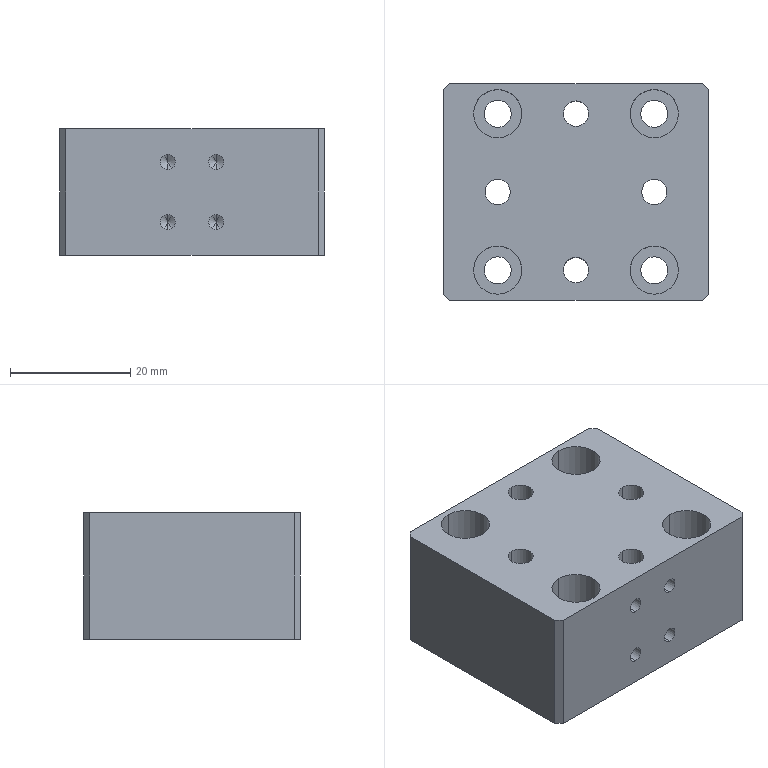NC program | NX | posted with a generic post | part box 44 x 36 x 21 mm
Whole program:
N10 G17 G21 G94 G90
(FLOOR_WALL_COPY , TOOL : D63)
N12 T01 M6
N14 G54
N16 G17 G0 G90 X-56.5 Y0. B0. C0. S6500 M3
N18 G43 Z30. H1
N20 Z6.
N22 G94 G1 Z3. F1250.
N24 X-53.5
N26 X53.5
N28 X56.5
N30 Z6.
N32 G0 Z30.
N34 X-56.5
N36 Z5.
N38 G1 Z2.
N40 X-53.5
N42 X53.5
N44 X56.5
N46 Z5.
N48 G0 Z30.
N50 X-56.5
N52 Z4.
N54 G1 Z1.
N56 X-53.5
N58 X53.5
N60 X56.5
N62 Z4.
N64 G0 Z30.
N66 X-56.5
N68 Z3.
N70 G1 Z0.
N72 X-53.5
N74 X53.5
N76 X56.5
N78 Z3.
N80 G0 Z30.
N82 M5
(ZLEVEL_PROFILE_1_COPY_1_COPY , TOOL : D6A45)
N84 T07 M6
N86 G54
N88 G17 G0 G90 X13.042 Y13.081 B0. C0. S9500 M3
N90 G43 Z30. H7
N92 Z0.
N94 G94 G1 Z-1. F1000.
N96 X13.52 Y13.991
N98 G3 X13. Y14.291 R0.6
N100 G1 X12.997
N102 G3 X11.709 Y12.997 R1.291
N104 X13. Y14.291 R-1.291
N106 X12.48 Y13.991 R0.6
N108 G1 X12.958 Y13.081
N110 Z0.
N112 G0 Z30.
N114 X-12.958
N116 Z0.
N118 G1 Z-1.
N120 X-12.48 Y13.991
N122 G3 X-13. Y14.291 R0.6
N124 X-14.291 Y13. R1.291
N126 X-13. Y14.291 R-1.291
N128 X-13.52 Y13.991 R0.6
N130 G1 X-13.042 Y13.081
N132 Z0.
N134 G0 Z30.
N136 X14.141 Y0.
N138 Z1.
N140 G1 Z-1.
N142 G3 X13. Y1.141 R1.141
N144 X14.141 Y0. R-1.141
N146 X13.841 Y0.52 R0.6
N148 G1 Z0.
N150 G0 Z30.
N152 X-14.141 Y0.
N154 Z1.
N156 G1 Z-1.
N158 G3 X-13. Y-1.141 R1.141
N160 X-14.141 Y0. R-1.141
N162 X-13.841 Y-0.52 R0.6
N164 G1 Z0.
N166 G0 Z30.
N168 X0. Y-14.141
N170 Z1.
N172 G1 Z-1.
N174 X0.005
N176 G3 X1.141 Y-12.995 R1.141
N178 X0. Y-14.141 R-1.141
N180 X0.52 Y-13.841 R0.6
N182 G1 Z0.
N184 G0 Z30.
N186 X12.958 Y-13.081
N188 Z0.
N190 G1 Z-1.
N192 X12.48 Y-13.991
N194 G3 X13. Y-14.291 R0.6
N196 X14.291 Y-13. R1.291
N198 X13. Y-14.291 R-1.291
N200 X13.52 Y-13.991 R0.6
N202 G1 X13.042 Y-13.081
N204 Z0.
N206 G0 Z30.
N208 X-13.042
N210 Z0.
N212 G1 Z-1.
N214 X-13.52 Y-13.991
N216 G3 X-13. Y-14.291 R0.6
N218 G1 X-12.997
N220 G3 X-11.709 Y-12.997 R1.291
N222 X-13. Y-14.291 R-1.291
N224 X-12.48 Y-13.991 R0.6
N226 G1 X-12.958 Y-13.081
N228 Z0.
N230 G0 Z30.
N232 X0. Y14.141
N234 Z1.
N236 G1 Z-1.
N238 X-0.008
N240 G3 X-1.141 Y12.992 R1.141
N242 X0. Y14.141 R-1.141
N244 X-0.52 Y13.841 R0.6
N246 G1 Z0.
N248 G0 Z30.
N250 X-21.921 Y19.952
N252 Z0.
N254 G1 Z-1.
N256 X-21.52 Y19.259
N258 G3 X-21.001 Y18.959 R0.6
N260 G1 X21.001
N262 G2 X21.677 Y18.678 R0.957
N264 G1 X22.678 Y17.677
N266 G2 X22.959 Y17.001 R0.956
N268 G1 Y-17.001
N270 G2 X22.678 Y-17.677 R0.956
N272 G1 X21.677 Y-18.678
N274 G2 X21.001 Y-18.959 R0.957
N276 G1 X-21.001
N278 G2 X-21.677 Y-18.678 R0.957
N280 G1 X-22.678 Y-17.677
N282 G2 X-22.959 Y-17.001 R0.956
N284 G1 Y17.001
N286 G2 X-22.678 Y17.677 R0.956
N288 G1 X-21.677 Y18.678
N290 G2 X-21.001 Y18.959 R0.957
N292 G3 X-20.481 Y19.259 R0.6
N294 G1 X-19.962 Y20.159
N296 Z0.
N298 G0 Z30.
N300 M5
N302 M2